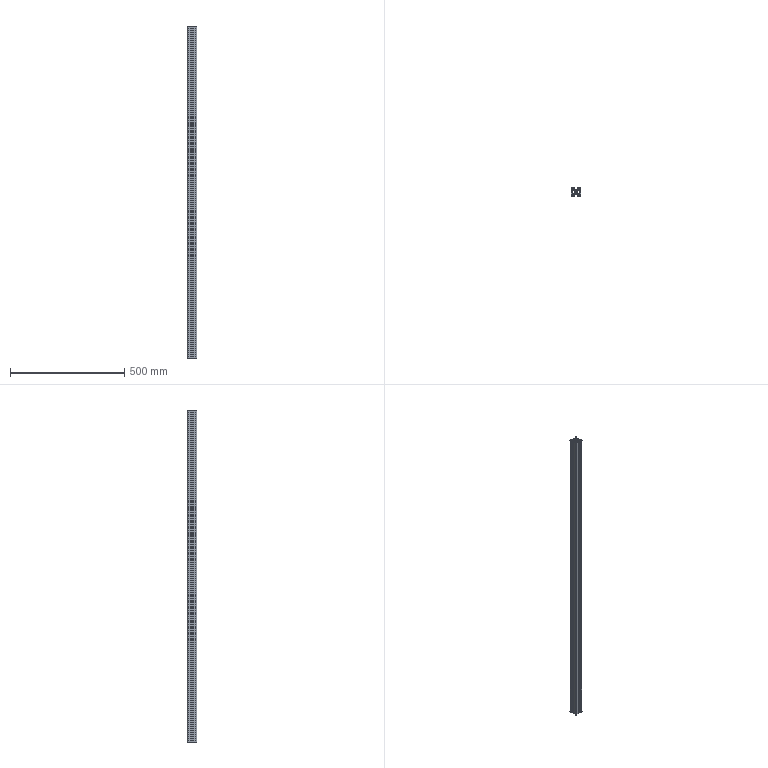Part | STEP file | 1.6米HFS8-4040-2150 | 1 solid | 111 faces | box 40 x 40 x 1450 mm | volume 901973 mm3 | plane 74 | cylinder 37 | commonest cylinder face diameters 2 x28 10.5 x5 6 x4